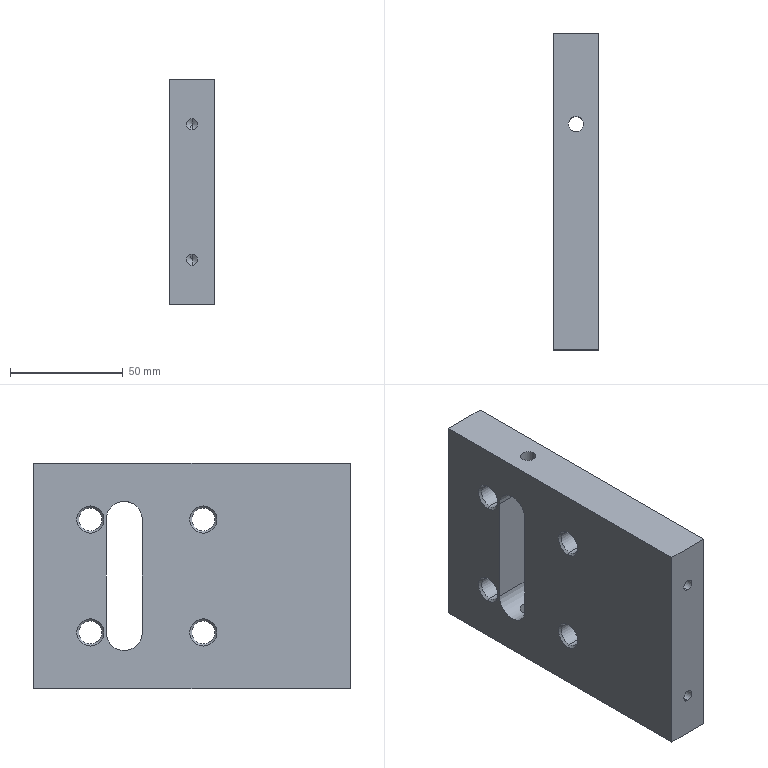Part | SolidWorks | features HoleWzd 4, Extrusion 1, ICE 1 | 1 solid | 47 faces | box 20 x 140 x 100 mm | volume 250918 mm3 | cylinder 23 | cone 16 | plane 8 | commonest cylinder face diameters 5 x8 10.2 x8 6.8 x4 16 x3
STEP:
#1=CARTESIAN_POINT('',(10.,55.,-32.5));
#2=VERTEX_POINT('',#1);
#3=CARTESIAN_POINT('',(10.,55.,-27.5));
#4=VERTEX_POINT('',#3);
#5=CARTESIAN_POINT('',(10.,55.,-30.));
#6=DIRECTION('',(0.,1.,0.));
#7=DIRECTION('',(0.,0.,1.));
#8=AXIS2_PLACEMENT_3D('',#5,#6,#7);
#9=CIRCLE('',#8,2.5);
#10=EDGE_CURVE('',#2,#4,#9,.T.);
#11=ORIENTED_EDGE('',*,*,#10,.F.);
#12=CARTESIAN_POINT('',(10.,70.,-32.5));
#13=VERTEX_POINT('',#12);
#14=CARTESIAN_POINT('',(10.,70.,-32.5));
#15=DIRECTION('',(0.,1.,0.));
#16=VECTOR('',#15,1000.);
#17=LINE('',#14,#16);
#18=EDGE_CURVE('',#2,#13,#17,.T.);
#19=ORIENTED_EDGE('',*,*,#18,.T.);
#20=CARTESIAN_POINT('',(10.,70.,-27.5));
#21=VERTEX_POINT('',#20);
#22=CARTESIAN_POINT('',(10.,70.,-30.));
#23=DIRECTION('',(0.,1.,0.));
#24=DIRECTION('',(0.,0.,1.));
#25=AXIS2_PLACEMENT_3D('',#22,#23,#24);
#26=CIRCLE('',#25,2.5);
#27=EDGE_CURVE('',#13,#21,#26,.T.);
#28=ORIENTED_EDGE('',*,*,#27,.T.);
#29=CARTESIAN_POINT('',(10.,70.,-27.5));
#30=DIRECTION('',(0.,1.,0.));
#31=VECTOR('',#30,1000.);
#32=LINE('',#29,#31);
#33=EDGE_CURVE('',#4,#21,#32,.T.);
#34=ORIENTED_EDGE('',*,*,#33,.F.);
#35=EDGE_LOOP('',(#11,#19,#28,#34));
#36=FACE_OUTER_BOUND('',#35,.T.);
#37=CARTESIAN_POINT('',(10.,70.,-30.));
#38=DIRECTION('',(0.,1.,0.));
#39=DIRECTION('',(0.,0.,1.));
#40=AXIS2_PLACEMENT_3D('',#37,#38,#39);
#41=CYLINDRICAL_SURFACE('',#40,2.5);
#42=ADVANCED_FACE('',(#36),#41,.F.);
#43=CARTESIAN_POINT('',(10.,53.498,-30.));
#44=VERTEX_POINT('',#43);
#45=CARTESIAN_POINT('',(10.,55.,-27.5));
#46=DIRECTION('',(0.,0.515,0.8572));
#47=VECTOR('',#46,1000.);
#48=LINE('',#45,#47);
#49=EDGE_CURVE('',#44,#4,#48,.T.);
#50=ORIENTED_EDGE('',*,*,#49,.F.);
#51=CARTESIAN_POINT('',(10.,55.,-32.5));
#52=DIRECTION('',(0.,0.515,-0.8572));
#53=VECTOR('',#52,1000.);
#54=LINE('',#51,#53);
#55=EDGE_CURVE('',#44,#2,#54,.T.);
#56=ORIENTED_EDGE('',*,*,#55,.T.);
#57=ORIENTED_EDGE('',*,*,#10,.T.);
#58=EDGE_LOOP('',(#50,#56,#57));
#59=FACE_OUTER_BOUND('',#58,.T.);
#60=CARTESIAN_POINT('',(10.,55.,-30.));
#61=DIRECTION('',(0.,1.,0.));
#62=DIRECTION('',(0.,0.,1.));
#63=AXIS2_PLACEMENT_3D('',#60,#61,#62);
#64=CONICAL_SURFACE('',#63,2.5,1.03);
#65=ADVANCED_FACE('',(#59),#64,.F.);
#66=CARTESIAN_POINT('',(10.,55.,27.5));
#67=VERTEX_POINT('',#66);
#68=CARTESIAN_POINT('',(10.,55.,32.5));
#69=VERTEX_POINT('',#68);
#70=CARTESIAN_POINT('',(10.,55.,30.));
#71=DIRECTION('',(0.,1.,0.));
#72=DIRECTION('',(0.,0.,1.));
#73=AXIS2_PLACEMENT_3D('',#70,#71,#72);
#74=CIRCLE('',#73,2.5);
#75=EDGE_CURVE('',#67,#69,#74,.T.);
#76=ORIENTED_EDGE('',*,*,#75,.F.);
#77=CARTESIAN_POINT('',(10.,70.,27.5));
#78=VERTEX_POINT('',#77);
#79=CARTESIAN_POINT('',(10.,70.,27.5));
#80=DIRECTION('',(0.,1.,0.));
#81=VECTOR('',#80,1000.);
#82=LINE('',#79,#81);
#83=EDGE_CURVE('',#67,#78,#82,.T.);
#84=ORIENTED_EDGE('',*,*,#83,.T.);
#85=CARTESIAN_POINT('',(10.,70.,32.5));
#86=VERTEX_POINT('',#85);
#87=CARTESIAN_POINT('',(10.,70.,30.));
#88=DIRECTION('',(0.,1.,0.));
#89=DIRECTION('',(0.,0.,1.));
#90=AXIS2_PLACEMENT_3D('',#87,#88,#89);
#91=CIRCLE('',#90,2.5);
#92=EDGE_CURVE('',#78,#86,#91,.T.);
#93=ORIENTED_EDGE('',*,*,#92,.T.);
#94=CARTESIAN_POINT('',(10.,70.,32.5));
#95=DIRECTION('',(0.,1.,0.));
#96=VECTOR('',#95,1000.);
#97=LINE('',#94,#96);
#98=EDGE_CURVE('',#69,#86,#97,.T.);
#99=ORIENTED_EDGE('',*,*,#98,.F.);
#100=EDGE_LOOP('',(#76,#84,#93,#99));
#101=FACE_OUTER_BOUND('',#100,.T.);
#102=CARTESIAN_POINT('',(10.,70.,30.));
#103=DIRECTION('',(0.,1.,0.));
#104=DIRECTION('',(0.,0.,1.));
#105=AXIS2_PLACEMENT_3D('',#102,#103,#104);
#106=CYLINDRICAL_SURFACE('',#105,2.5);
#107=ADVANCED_FACE('',(#101),#106,.F.);
#108=CARTESIAN_POINT('',(10.,53.498,30.));
#109=VERTEX_POINT('',#108);
#110=CARTESIAN_POINT('',(10.,55.,32.5));
#111=DIRECTION('',(0.,0.515,0.8572));
#112=VECTOR('',#111,1000.);
#113=LINE('',#110,#112);
#114=EDGE_CURVE('',#109,#69,#113,.T.);
#115=ORIENTED_EDGE('',*,*,#114,.F.);
#116=CARTESIAN_POINT('',(10.,55.,27.5));
#117=DIRECTION('',(0.,0.515,-0.8572));
#118=VECTOR('',#117,1000.);
#119=LINE('',#116,#118);
#120=EDGE_CURVE('',#109,#67,#119,.T.);
#121=ORIENTED_EDGE('',*,*,#120,.T.);
#122=ORIENTED_EDGE('',*,*,#75,.T.);
#123=EDGE_LOOP('',(#115,#121,#122));
#124=FACE_OUTER_BOUND('',#123,.T.);
#125=CARTESIAN_POINT('',(10.,55.,30.));
#126=DIRECTION('',(0.,1.,0.));
#127=DIRECTION('',(0.,0.,1.));
#128=AXIS2_PLACEMENT_3D('',#125,#126,#127);
#129=CONICAL_SURFACE('',#128,2.5,1.03);
#130=ADVANCED_FACE('',(#124),#129,.F.);
#131=CARTESIAN_POINT('',(0.925,45.,-30.1));
#132=VERTEX_POINT('',#131);
#133=CARTESIAN_POINT('',(0.925,45.,-19.9));
#134=VERTEX_POINT('',#133);
#135=CARTESIAN_POINT('',(0.925,45.,-25.));
#136=DIRECTION('',(-1.,0.,0.));
#137=DIRECTION('',(0.,0.,1.));
#138=AXIS2_PLACEMENT_3D('',#135,#136,#137);
#139=CIRCLE('',#138,5.1);
#140=EDGE_CURVE('',#132,#134,#139,.T.);
#141=ORIENTED_EDGE('',*,*,#140,.F.);
#142=CARTESIAN_POINT('',(0.,45.,-31.025));
#143=VERTEX_POINT('',#142);
#144=CARTESIAN_POINT('',(0.,45.,-31.025));
#145=DIRECTION('',(-0.7071,0.,-0.7071));
#146=VECTOR('',#145,1000.);
#147=LINE('',#144,#146);
#148=EDGE_CURVE('',#132,#143,#147,.T.);
#149=ORIENTED_EDGE('',*,*,#148,.T.);
#150=CARTESIAN_POINT('',(0.,45.,-18.975));
#151=VERTEX_POINT('',#150);
#152=CARTESIAN_POINT('',(0.,45.,-25.));
#153=DIRECTION('',(-1.,0.,0.));
#154=DIRECTION('',(0.,0.,1.));
#155=AXIS2_PLACEMENT_3D('',#152,#153,#154);
#156=CIRCLE('',#155,6.025);
#157=EDGE_CURVE('',#143,#151,#156,.T.);
#158=ORIENTED_EDGE('',*,*,#157,.T.);
#159=CARTESIAN_POINT('',(0.,45.,-18.975));
#160=DIRECTION('',(-0.7071,0.,0.7071));
#161=VECTOR('',#160,1000.);
#162=LINE('',#159,#161);
#163=EDGE_CURVE('',#134,#151,#162,.T.);
#164=ORIENTED_EDGE('',*,*,#163,.F.);
#165=EDGE_LOOP('',(#141,#149,#158,#164));
#166=FACE_OUTER_BOUND('',#165,.T.);
#167=CARTESIAN_POINT('',(0.,45.,-25.));
#168=DIRECTION('',(-1.,0.,0.));
#169=DIRECTION('',(0.,0.,1.));
#170=AXIS2_PLACEMENT_3D('',#167,#168,#169);
#171=CONICAL_SURFACE('',#170,6.025,0.7854);
#172=ADVANCED_FACE('',(#166),#171,.F.);
#173=CARTESIAN_POINT('',(20.,45.,-30.1));
#174=VERTEX_POINT('',#173);
#175=CARTESIAN_POINT('',(20.,45.,-19.9));
#176=VERTEX_POINT('',#175);
#177=CARTESIAN_POINT('',(20.,45.,-25.));
#178=DIRECTION('',(-1.,0.,0.));
#179=DIRECTION('',(0.,0.,1.));
#180=AXIS2_PLACEMENT_3D('',#177,#178,#179);
#181=CIRCLE('',#180,5.1);
#182=EDGE_CURVE('',#174,#176,#181,.T.);
#183=ORIENTED_EDGE('',*,*,#182,.F.);
#184=CARTESIAN_POINT('',(0.,45.,-30.1));
#185=DIRECTION('',(-1.,0.,0.));
#186=VECTOR('',#185,1000.);
#187=LINE('',#184,#186);
#188=EDGE_CURVE('',#174,#132,#187,.T.);
#189=ORIENTED_EDGE('',*,*,#188,.T.);
#190=ORIENTED_EDGE('',*,*,#140,.T.);
#191=CARTESIAN_POINT('',(0.,45.,-19.9));
#192=DIRECTION('',(-1.,0.,0.));
#193=VECTOR('',#192,1000.);
#194=LINE('',#191,#193);
#195=EDGE_CURVE('',#176,#134,#194,.T.);
#196=ORIENTED_EDGE('',*,*,#195,.F.);
#197=EDGE_LOOP('',(#183,#189,#190,#196));
#198=FACE_OUTER_BOUND('',#197,.T.);
#199=CARTESIAN_POINT('',(0.,45.,-25.));
#200=DIRECTION('',(-1.,0.,0.));
#201=DIRECTION('',(0.,0.,1.));
#202=AXIS2_PLACEMENT_3D('',#199,#200,#201);
#203=CYLINDRICAL_SURFACE('',#202,5.1);
#204=ADVANCED_FACE('',(#198),#203,.F.);
#205=CARTESIAN_POINT('',(0.925,45.,19.9));
#206=VERTEX_POINT('',#205);
#207=CARTESIAN_POINT('',(0.925,45.,30.1));
#208=VERTEX_POINT('',#207);
#209=CARTESIAN_POINT('',(0.925,45.,25.));
#210=DIRECTION('',(-1.,0.,0.));
#211=DIRECTION('',(0.,0.,1.));
#212=AXIS2_PLACEMENT_3D('',#209,#210,#211);
#213=CIRCLE('',#212,5.1);
#214=EDGE_CURVE('',#206,#208,#213,.T.);
#215=ORIENTED_EDGE('',*,*,#214,.F.);
#216=CARTESIAN_POINT('',(0.,45.,18.975));
#217=VERTEX_POINT('',#216);
#218=CARTESIAN_POINT('',(0.,45.,18.975));
#219=DIRECTION('',(-0.7071,0.,-0.7071));
#220=VECTOR('',#219,1000.);
#221=LINE('',#218,#220);
#222=EDGE_CURVE('',#206,#217,#221,.T.);
#223=ORIENTED_EDGE('',*,*,#222,.T.);
#224=CARTESIAN_POINT('',(0.,45.,31.025));
#225=VERTEX_POINT('',#224);
#226=CARTESIAN_POINT('',(0.,45.,25.));
#227=DIRECTION('',(-1.,0.,0.));
#228=DIRECTION('',(0.,0.,1.));
#229=AXIS2_PLACEMENT_3D('',#226,#227,#228);
#230=CIRCLE('',#229,6.025);
#231=EDGE_CURVE('',#217,#225,#230,.T.);
#232=ORIENTED_EDGE('',*,*,#231,.T.);
#233=CARTESIAN_POINT('',(0.,45.,31.025));
#234=DIRECTION('',(-0.7071,0.,0.7071));
#235=VECTOR('',#234,1000.);
#236=LINE('',#233,#235);
#237=EDGE_CURVE('',#208,#225,#236,.T.);
#238=ORIENTED_EDGE('',*,*,#237,.F.);
#239=EDGE_LOOP('',(#215,#223,#232,#238));
#240=FACE_OUTER_BOUND('',#239,.T.);
#241=CARTESIAN_POINT('',(0.,45.,25.));
#242=DIRECTION('',(-1.,0.,0.));
#243=DIRECTION('',(0.,0.,1.));
#244=AXIS2_PLACEMENT_3D('',#241,#242,#243);
#245=CONICAL_SURFACE('',#244,6.025,0.7854);
#246=ADVANCED_FACE('',(#240),#245,.F.);
#247=CARTESIAN_POINT('',(20.,45.,19.9));
#248=VERTEX_POINT('',#247);
#249=CARTESIAN_POINT('',(20.,45.,30.1));
#250=VERTEX_POINT('',#249);
#251=CARTESIAN_POINT('',(20.,45.,25.));
#252=DIRECTION('',(-1.,0.,0.));
#253=DIRECTION('',(0.,0.,1.));
#254=AXIS2_PLACEMENT_3D('',#251,#252,#253);
#255=CIRCLE('',#254,5.1);
#256=EDGE_CURVE('',#248,#250,#255,.T.);
#257=ORIENTED_EDGE('',*,*,#256,.F.);
#258=CARTESIAN_POINT('',(0.,45.,19.9));
#259=DIRECTION('',(-1.,0.,0.));
#260=VECTOR('',#259,1000.);
#261=LINE('',#258,#260);
#262=EDGE_CURVE('',#248,#206,#261,.T.);
#263=ORIENTED_EDGE('',*,*,#262,.T.);
#264=ORIENTED_EDGE('',*,*,#214,.T.);
#265=CARTESIAN_POINT('',(0.,45.,30.1));
#266=DIRECTION('',(-1.,0.,0.));
#267=VECTOR('',#266,1000.);
#268=LINE('',#265,#267);
#269=EDGE_CURVE('',#250,#208,#268,.T.);
#270=ORIENTED_EDGE('',*,*,#269,.F.);
#271=EDGE_LOOP('',(#257,#263,#264,#270));
#272=FACE_OUTER_BOUND('',#271,.T.);
#273=CARTESIAN_POINT('',(0.,45.,25.));
#274=DIRECTION('',(-1.,0.,0.));
#275=DIRECTION('',(0.,0.,1.));
#276=AXIS2_PLACEMENT_3D('',#273,#274,#275);
#277=CYLINDRICAL_SURFACE('',#276,5.1);
#278=ADVANCED_FACE('',(#272),#277,.F.);
#279=CARTESIAN_POINT('',(0.925,-5.,-30.1));
#280=VERTEX_POINT('',#279);
#281=CARTESIAN_POINT('',(0.925,-5.,-19.9));
#282=VERTEX_POINT('',#281);
#283=CARTESIAN_POINT('',(0.925,-5.,-25.));
#284=DIRECTION('',(-1.,0.,0.));
#285=DIRECTION('',(0.,0.,1.));
#286=AXIS2_PLACEMENT_3D('',#283,#284,#285);
#287=CIRCLE('',#286,5.1);
#288=EDGE_CURVE('',#280,#282,#287,.T.);
#289=ORIENTED_EDGE('',*,*,#288,.F.);
#290=CARTESIAN_POINT('',(0.,-5.,-31.025));
#291=VERTEX_POINT('',#290);
#292=CARTESIAN_POINT('',(0.,-5.,-31.025));
#293=DIRECTION('',(-0.7071,0.,-0.7071));
#294=VECTOR('',#293,1000.);
#295=LINE('',#292,#294);
#296=EDGE_CURVE('',#280,#291,#295,.T.);
#297=ORIENTED_EDGE('',*,*,#296,.T.);
#298=CARTESIAN_POINT('',(0.,-5.,-18.975));
#299=VERTEX_POINT('',#298);
#300=CARTESIAN_POINT('',(0.,-5.,-25.));
#301=DIRECTION('',(-1.,0.,0.));
#302=DIRECTION('',(0.,0.,1.));
#303=AXIS2_PLACEMENT_3D('',#300,#301,#302);
#304=CIRCLE('',#303,6.025);
#305=EDGE_CURVE('',#291,#299,#304,.T.);
#306=ORIENTED_EDGE('',*,*,#305,.T.);
#307=CARTESIAN_POINT('',(0.,-5.,-18.975));
#308=DIRECTION('',(-0.7071,0.,0.7071));
#309=VECTOR('',#308,1000.);
#310=LINE('',#307,#309);
#311=EDGE_CURVE('',#282,#299,#310,.T.);
#312=ORIENTED_EDGE('',*,*,#311,.F.);
#313=EDGE_LOOP('',(#289,#297,#306,#312));
#314=FACE_OUTER_BOUND('',#313,.T.);
#315=CARTESIAN_POINT('',(0.,-5.,-25.));
#316=DIRECTION('',(-1.,0.,0.));
#317=DIRECTION('',(0.,0.,1.));
#318=AXIS2_PLACEMENT_3D('',#315,#316,#317);
#319=CONICAL_SURFACE('',#318,6.025,0.7854);
#320=ADVANCED_FACE('',(#314),#319,.F.);
#321=CARTESIAN_POINT('',(20.,-5.,-30.1));
#322=VERTEX_POINT('',#321);
#323=CARTESIAN_POINT('',(20.,-5.,-19.9));
#324=VERTEX_POINT('',#323);
#325=CARTESIAN_POINT('',(20.,-5.,-25.));
#326=DIRECTION('',(-1.,0.,0.));
#327=DIRECTION('',(0.,0.,1.));
#328=AXIS2_PLACEMENT_3D('',#325,#326,#327);
#329=CIRCLE('',#328,5.1);
#330=EDGE_CURVE('',#322,#324,#329,.T.);
#331=ORIENTED_EDGE('',*,*,#330,.F.);
#332=CARTESIAN_POINT('',(0.,-5.,-30.1));
#333=DIRECTION('',(-1.,0.,0.));
#334=VECTOR('',#333,1000.);
#335=LINE('',#332,#334);
#336=EDGE_CURVE('',#322,#280,#335,.T.);
#337=ORIENTED_EDGE('',*,*,#336,.T.);
#338=ORIENTED_EDGE('',*,*,#288,.T.);
#339=CARTESIAN_POINT('',(0.,-5.,-19.9));
#340=DIRECTION('',(-1.,0.,0.));
#341=VECTOR('',#340,1000.);
#342=LINE('',#339,#341);
#343=EDGE_CURVE('',#324,#282,#342,.T.);
#344=ORIENTED_EDGE('',*,*,#343,.F.);
#345=EDGE_LOOP('',(#331,#337,#338,#344));
#346=FACE_OUTER_BOUND('',#345,.T.);
#347=CARTESIAN_POINT('',(0.,-5.,-25.));
#348=DIRECTION('',(-1.,0.,0.));
#349=DIRECTION('',(0.,0.,1.));
#350=AXIS2_PLACEMENT_3D('',#347,#348,#349);
#351=CYLINDRICAL_SURFACE('',#350,5.1);
#352=ADVANCED_FACE('',(#346),#351,.F.);
#353=CARTESIAN_POINT('',(0.925,-5.,19.9));
#354=VERTEX_POINT('',#353);
#355=CARTESIAN_POINT('',(0.925,-5.,30.1));
#356=VERTEX_POINT('',#355);
#357=CARTESIAN_POINT('',(0.925,-5.,25.));
#358=DIRECTION('',(-1.,0.,0.));
#359=DIRECTION('',(0.,0.,1.));
#360=AXIS2_PLACEMENT_3D('',#357,#358,#359);
#361=CIRCLE('',#360,5.1);
#362=EDGE_CURVE('',#354,#356,#361,.T.);
#363=ORIENTED_EDGE('',*,*,#362,.F.);
#364=CARTESIAN_POINT('',(0.,-5.,18.975));
#365=VERTEX_POINT('',#364);
#366=CARTESIAN_POINT('',(0.,-5.,18.975));
#367=DIRECTION('',(-0.7071,0.,-0.7071));
#368=VECTOR('',#367,1000.);
#369=LINE('',#366,#368);
#370=EDGE_CURVE('',#354,#365,#369,.T.);
#371=ORIENTED_EDGE('',*,*,#370,.T.);
#372=CARTESIAN_POINT('',(0.,-5.,31.025));
#373=VERTEX_POINT('',#372);
#374=CARTESIAN_POINT('',(0.,-5.,25.));
#375=DIRECTION('',(-1.,0.,0.));
#376=DIRECTION('',(0.,0.,1.));
#377=AXIS2_PLACEMENT_3D('',#374,#375,#376);
#378=CIRCLE('',#377,6.025);
#379=EDGE_CURVE('',#365,#373,#378,.T.);
#380=ORIENTED_EDGE('',*,*,#379,.T.);
#381=CARTESIAN_POINT('',(0.,-5.,31.025));
#382=DIRECTION('',(-0.7071,0.,0.7071));
#383=VECTOR('',#382,1000.);
#384=LINE('',#381,#383);
#385=EDGE_CURVE('',#356,#373,#384,.T.);
#386=ORIENTED_EDGE('',*,*,#385,.F.);
#387=EDGE_LOOP('',(#363,#371,#380,#386));
#388=FACE_OUTER_BOUND('',#387,.T.);
#389=CARTESIAN_POINT('',(0.,-5.,25.));
#390=DIRECTION('',(-1.,0.,0.));
#391=DIRECTION('',(0.,0.,1.));
#392=AXIS2_PLACEMENT_3D('',#389,#390,#391);
#393=CONICAL_SURFACE('',#392,6.025,0.7854);
#394=ADVANCED_FACE('',(#388),#393,.F.);
#395=CARTESIAN_POINT('',(20.,-5.,19.9));
#396=VERTEX_POINT('',#395);
#397=CARTESIAN_POINT('',(20.,-5.,30.1));
#398=VERTEX_POINT('',#397);
#399=CARTESIAN_POINT('',(20.,-5.,25.));
#400=DIRECTION('',(-1.,0.,0.));
#401=DIRECTION('',(0.,0.,1.));
#402=AXIS2_PLACEMENT_3D('',#399,#400,#401);
#403=CIRCLE('',#402,5.1);
#404=EDGE_CURVE('',#396,#398,#403,.T.);
#405=ORIENTED_EDGE('',*,*,#404,.F.);
#406=CARTESIAN_POINT('',(0.,-5.,19.9));
#407=DIRECTION('',(-1.,0.,0.));
#408=VECTOR('',#407,1000.);
#409=LINE('',#406,#408);
#410=EDGE_CURVE('',#396,#354,#409,.T.);
#411=ORIENTED_EDGE('',*,*,#410,.T.);
#412=ORIENTED_EDGE('',*,*,#362,.T.);
#413=CARTESIAN_POINT('',(0.,-5.,30.1));
#414=DIRECTION('',(-1.,0.,0.));
#415=VECTOR('',#414,1000.);
#416=LINE('',#413,#415);
#417=EDGE_CURVE('',#398,#356,#416,.T.);
#418=ORIENTED_EDGE('',*,*,#417,.F.);
#419=EDGE_LOOP('',(#405,#411,#412,#418));
#420=FACE_OUTER_BOUND('',#419,.T.);
#421=CARTESIAN_POINT('',(0.,-5.,25.));
#422=DIRECTION('',(-1.,0.,0.));
#423=DIRECTION('',(0.,0.,1.));
#424=AXIS2_PLACEMENT_3D('',#421,#422,#423);
#425=CYLINDRICAL_SURFACE('',#424,5.1);
#426=ADVANCED_FACE('',(#420),#425,.F.);
#427=CARTESIAN_POINT('',(6.6,30.,-50.));
#428=VERTEX_POINT('',#427);
#429=CARTESIAN_POINT('',(13.4,30.,-50.));
#430=VERTEX_POINT('',#429);
#431=CARTESIAN_POINT('',(10.,30.,-50.));
#432=DIRECTION('',(0.,0.,1.));
#433=DIRECTION('',(1.,0.,0.));
#434=AXIS2_PLACEMENT_3D('',#431,#432,#433);
#435=CIRCLE('',#434,3.4);
#436=EDGE_CURVE('',#428,#430,#435,.T.);
#437=ORIENTED_EDGE('',*,*,#436,.F.);
#438=CARTESIAN_POINT('',(6.6,30.,-33.));
#439=VERTEX_POINT('',#438);
#440=CARTESIAN_POINT('',(6.6,30.,50.));
#441=DIRECTION('',(0.,0.,1.));
#442=VECTOR('',#441,1000.);
#443=LINE('',#440,#442);
#444=EDGE_CURVE('',#428,#439,#443,.T.);
#445=ORIENTED_EDGE('',*,*,#444,.T.);
#446=CARTESIAN_POINT('',(13.4,30.,-33.));
#447=VERTEX_POINT('',#446);
#448=CARTESIAN_POINT('',(13.4,30.,-33.));
#449=CARTESIAN_POINT('',(13.4,29.772,-33.));
#450=CARTESIAN_POINT('',(13.377,29.549,-32.99));
#451=CARTESIAN_POINT('',(13.289,29.111,-32.953));
#452=CARTESIAN_POINT('',(13.223,28.893,-32.926));
#453=CARTESIAN_POINT('',(13.051,28.483,-32.858));
#454=CARTESIAN_POINT('',(12.946,28.288,-32.817));
#455=CARTESIAN_POINT('',(12.699,27.92,-32.727));
#456=CARTESIAN_POINT('',(12.557,27.749,-32.678));
#457=CARTESIAN_POINT('',(12.247,27.439,-32.581));
#458=CARTESIAN_POINT('',(12.077,27.299,-32.531));
#459=CARTESIAN_POINT('',(11.708,27.052,-32.438));
#460=CARTESIAN_POINT('',(11.514,26.948,-32.395));
#461=CARTESIAN_POINT('',(11.107,26.778,-32.323));
#462=CARTESIAN_POINT('',(10.89,26.711,-32.293));
#463=CARTESIAN_POINT('',(10.45,26.622,-32.252));
#464=CARTESIAN_POINT('',(10.227,26.6,-32.242));
#465=CARTESIAN_POINT('',(9.777,26.6,-32.241));
#466=CARTESIAN_POINT('',(9.549,26.623,-32.252));
#467=CARTESIAN_POINT('',(9.111,26.711,-32.293));
#468=CARTESIAN_POINT('',(8.896,26.776,-32.322));
#469=CARTESIAN_POINT('',(8.483,26.949,-32.396));
#470=CARTESIAN_POINT('',(8.289,27.054,-32.439));
#471=CARTESIAN_POINT('',(7.923,27.299,-32.531));
#472=CARTESIAN_POINT('',(7.75,27.441,-32.582));
#473=CARTESIAN_POINT('',(7.44,27.752,-32.679));
#474=CARTESIAN_POINT('',(7.301,27.921,-32.727));
#475=CARTESIAN_POINT('',(7.054,28.289,-32.817));
#476=CARTESIAN_POINT('',(6.948,28.486,-32.858));
#477=CARTESIAN_POINT('',(6.777,28.895,-32.926));
#478=CARTESIAN_POINT('',(6.711,29.108,-32.953));
#479=CARTESIAN_POINT('',(6.622,29.552,-32.991));
#480=CARTESIAN_POINT('',(6.6,29.776,-33.));
#481=CARTESIAN_POINT('',(6.6,30.,-33.));
#482=B_SPLINE_CURVE_WITH_KNOTS('',3,(#448,#449,#450,#451,#452,#453,#454,#455,#456,#457,#458,#459,#460,#461,#462,#463,#464,#465,#466,#467,#468,#469,#470,#471,#472,#473,#474,#475,#476,#477,#478,#479,#480,#481),.UNSPECIFIED.,.F.,.F.,(4,2,2,2,2,2,2,2,2,2,2,2,2,2,2,2,4),(0.,0.0006725,0.001345,0.002017,0.00269,0.003362,0.004035,0.004707,0.00538,0.006052,0.006725,0.007397,0.00807,0.008742,0.009415,0.01009,0.01076),.UNSPECIFIED.);
#483=EDGE_CURVE('',#447,#439,#482,.T.);
#484=ORIENTED_EDGE('',*,*,#483,.F.);
#485=CARTESIAN_POINT('',(13.4,30.,50.));
#486=DIRECTION('',(0.,0.,1.));
#487=VECTOR('',#486,1000.);
#488=LINE('',#485,#487);
#489=EDGE_CURVE('',#430,#447,#488,.T.);
#490=ORIENTED_EDGE('',*,*,#489,.F.);
#491=EDGE_LOOP('',(#437,#445,#484,#490));
#492=FACE_OUTER_BOUND('',#491,.T.);
#493=CARTESIAN_POINT('',(10.,30.,50.));
#494=DIRECTION('',(0.,0.,1.));
#495=DIRECTION('',(1.,0.,0.));
#496=AXIS2_PLACEMENT_3D('',#493,#494,#495);
#497=CYLINDRICAL_SURFACE('',#496,3.4);
#498=ADVANCED_FACE('',(#492),#497,.F.);
#499=CARTESIAN_POINT('',(6.6,30.,33.));
#500=VERTEX_POINT('',#499);
#501=CARTESIAN_POINT('',(13.4,30.,33.));
#502=VERTEX_POINT('',#501);
#503=CARTESIAN_POINT('',(6.6,30.,33.));
#504=CARTESIAN_POINT('',(6.6,29.776,33.));
#505=CARTESIAN_POINT('',(6.623,29.549,32.99));
#506=CARTESIAN_POINT('',(6.711,29.108,32.953));
#507=CARTESIAN_POINT('',(6.777,28.895,32.926));
#508=CARTESIAN_POINT('',(6.949,28.483,32.858));
#509=CARTESIAN_POINT('',(7.055,28.286,32.816));
#510=CARTESIAN_POINT('',(7.301,27.921,32.727));
#511=CARTESIAN_POINT('',(7.442,27.75,32.679));
#512=CARTESIAN_POINT('',(7.754,27.438,32.58));
#513=CARTESIAN_POINT('',(7.924,27.299,32.531));
#514=CARTESIAN_POINT('',(8.288,27.054,32.439));
#515=CARTESIAN_POINT('',(8.486,26.947,32.395));
#516=CARTESIAN_POINT('',(8.896,26.777,32.322));
#517=CARTESIAN_POINT('',(9.108,26.712,32.293));
#518=CARTESIAN_POINT('',(9.547,26.623,32.252));
#519=CARTESIAN_POINT('',(9.775,26.6,32.242));
#520=CARTESIAN_POINT('',(10.223,26.6,32.242));
#521=CARTESIAN_POINT('',(10.446,26.622,32.252));
#522=CARTESIAN_POINT('',(10.891,26.711,32.293));
#523=CARTESIAN_POINT('',(11.104,26.776,32.322));
#524=CARTESIAN_POINT('',(11.513,26.947,32.395));
#525=CARTESIAN_POINT('',(11.711,27.054,32.439));
#526=CARTESIAN_POINT('',(12.077,27.299,32.531));
#527=CARTESIAN_POINT('',(12.247,27.438,32.581));
#528=CARTESIAN_POINT('',(12.559,27.75,32.679));
#529=CARTESIAN_POINT('',(12.7,27.922,32.728));
#530=CARTESIAN_POINT('',(12.945,28.286,32.817));
#531=CARTESIAN_POINT('',(13.05,28.482,32.857));
#532=CARTESIAN_POINT('',(13.223,28.896,32.926));
#533=CARTESIAN_POINT('',(13.289,29.108,32.953));
#534=CARTESIAN_POINT('',(13.377,29.546,32.99));
#535=CARTESIAN_POINT('',(13.4,29.773,33.));
#536=CARTESIAN_POINT('',(13.4,30.,33.));
#537=B_SPLINE_CURVE_WITH_KNOTS('',3,(#503,#504,#505,#506,#507,#508,#509,#510,#511,#512,#513,#514,#515,#516,#517,#518,#519,#520,#521,#522,#523,#524,#525,#526,#527,#528,#529,#530,#531,#532,#533,#534,#535,#536),.UNSPECIFIED.,.F.,.F.,(4,2,2,2,2,2,2,2,2,2,2,2,2,2,2,2,4),(0.01076,0.01143,0.0121,0.01278,0.01345,0.01412,0.01479,0.01546,0.01613,0.01681,0.01748,0.01815,0.01882,0.01949,0.02017,0.02084,0.02151),.UNSPECIFIED.);
#538=EDGE_CURVE('',#500,#502,#537,.T.);
#539=ORIENTED_EDGE('',*,*,#538,.F.);
#540=CARTESIAN_POINT('',(6.6,30.,50.));
#541=VERTEX_POINT('',#540);
#542=CARTESIAN_POINT('',(6.6,30.,50.));
#543=DIRECTION('',(0.,0.,1.));
#544=VECTOR('',#543,1000.);
#545=LINE('',#542,#544);
#546=EDGE_CURVE('',#500,#541,#545,.T.);
#547=ORIENTED_EDGE('',*,*,#546,.T.);
#548=CARTESIAN_POINT('',(13.4,30.,50.));
#549=VERTEX_POINT('',#548);
#550=CARTESIAN_POINT('',(10.,30.,50.));
#551=DIRECTION('',(0.,0.,1.));
#552=DIRECTION('',(1.,0.,0.));
#553=AXIS2_PLACEMENT_3D('',#550,#551,#552);
#554=CIRCLE('',#553,3.4);
#555=EDGE_CURVE('',#541,#549,#554,.T.);
#556=ORIENTED_EDGE('',*,*,#555,.T.);
#557=CARTESIAN_POINT('',(13.4,30.,50.));
#558=DIRECTION('',(0.,0.,1.));
#559=VECTOR('',#558,1000.);
#560=LINE('',#557,#559);
#561=EDGE_CURVE('',#502,#549,#560,.T.);
#562=ORIENTED_EDGE('',*,*,#561,.F.);
#563=EDGE_LOOP('',(#539,#547,#556,#562));
#564=FACE_OUTER_BOUND('',#563,.T.);
#565=CARTESIAN_POINT('',(10.,30.,50.));
#566=DIRECTION('',(0.,0.,1.));
#567=DIRECTION('',(1.,0.,0.));
#568=AXIS2_PLACEMENT_3D('',#565,#566,#567);
#569=CYLINDRICAL_SURFACE('',#568,3.4);
#570=ADVANCED_FACE('',(#564),#569,.F.);
#571=CARTESIAN_POINT('',(20.,30.,33.));
#572=VERTEX_POINT('',#571);
#573=CARTESIAN_POINT('',(20.,38.,25.));
#574=VERTEX_POINT('',#573);
#575=CARTESIAN_POINT('',(20.,30.,25.));
#576=DIRECTION('',(-1.,0.,0.));
#577=DIRECTION('',(0.,0.,1.));
#578=AXIS2_PLACEMENT_3D('',#575,#576,#577);
#579=CIRCLE('',#578,8.);
#580=EDGE_CURVE('',#572,#574,#579,.T.);
#581=ORIENTED_EDGE('',*,*,#580,.F.);
#582=CARTESIAN_POINT('',(20.,30.,33.));
#583=DIRECTION('',(-1.,0.,0.));
#584=VECTOR('',#583,1000.);
#585=LINE('',#582,#584);
#586=EDGE_CURVE('',#572,#502,#585,.T.);
#587=ORIENTED_EDGE('',*,*,#586,.T.);
#588=CARTESIAN_POINT('',(13.4,30.,33.));
#589=CARTESIAN_POINT('',(13.4,30.228,33.));
#590=CARTESIAN_POINT('',(13.377,30.451,32.99));
#591=CARTESIAN_POINT('',(13.289,30.889,32.953));
#592=CARTESIAN_POINT('',(13.223,31.107,32.926));
#593=CARTESIAN_POINT('',(13.051,31.517,32.858));
#594=CARTESIAN_POINT('',(12.946,31.712,32.817));
#595=CARTESIAN_POINT('',(12.699,32.08,32.727));
#596=CARTESIAN_POINT('',(12.557,32.251,32.678));
#597=CARTESIAN_POINT('',(12.247,32.561,32.581));
#598=CARTESIAN_POINT('',(12.077,32.701,32.531));
#599=CARTESIAN_POINT('',(11.708,32.948,32.438));
#600=CARTESIAN_POINT('',(11.514,33.052,32.395));
#601=CARTESIAN_POINT('',(11.107,33.222,32.323));
#602=CARTESIAN_POINT('',(10.89,33.289,32.293));
#603=CARTESIAN_POINT('',(10.45,33.378,32.252));
#604=CARTESIAN_POINT('',(10.227,33.4,32.242));
#605=CARTESIAN_POINT('',(9.777,33.4,32.241));
#606=CARTESIAN_POINT('',(9.549,33.377,32.252));
#607=CARTESIAN_POINT('',(9.111,33.289,32.293));
#608=CARTESIAN_POINT('',(8.896,33.224,32.322));
#609=CARTESIAN_POINT('',(8.483,33.051,32.396));
#610=CARTESIAN_POINT('',(8.289,32.946,32.439));
#611=CARTESIAN_POINT('',(7.923,32.701,32.531));
#612=CARTESIAN_POINT('',(7.75,32.559,32.582));
#613=CARTESIAN_POINT('',(7.44,32.248,32.679));
#614=CARTESIAN_POINT('',(7.301,32.079,32.727));
#615=CARTESIAN_POINT('',(7.054,31.711,32.817));
#616=CARTESIAN_POINT('',(6.948,31.514,32.858));
#617=CARTESIAN_POINT('',(6.777,31.105,32.926));
#618=CARTESIAN_POINT('',(6.711,30.892,32.953));
#619=CARTESIAN_POINT('',(6.622,30.448,32.991));
#620=CARTESIAN_POINT('',(6.6,30.224,33.));
#621=CARTESIAN_POINT('',(6.6,30.,33.));
#622=B_SPLINE_CURVE_WITH_KNOTS('',3,(#588,#589,#590,#591,#592,#593,#594,#595,#596,#597,#598,#599,#600,#601,#602,#603,#604,#605,#606,#607,#608,#609,#610,#611,#612,#613,#614,#615,#616,#617,#618,#619,#620,#621),.UNSPECIFIED.,.F.,.F.,(4,2,2,2,2,2,2,2,2,2,2,2,2,2,2,2,4),(0.,0.0006725,0.001345,0.002017,0.00269,0.003362,0.004035,0.004707,0.00538,0.006052,0.006725,0.007397,0.00807,0.008742,0.009415,0.01009,0.01076),.UNSPECIFIED.);
#623=EDGE_CURVE('',#502,#500,#622,.T.);
#624=ORIENTED_EDGE('',*,*,#623,.T.);
#625=CARTESIAN_POINT('',(0.,30.,33.));
#626=VERTEX_POINT('',#625);
#627=CARTESIAN_POINT('',(20.,30.,33.));
#628=DIRECTION('',(-1.,0.,0.));
#629=VECTOR('',#628,1000.);
#630=LINE('',#627,#629);
#631=EDGE_CURVE('',#500,#626,#630,.T.);
#632=ORIENTED_EDGE('',*,*,#631,.T.);
#633=CARTESIAN_POINT('',(0.,38.,25.));
#634=VERTEX_POINT('',#633);
#635=CARTESIAN_POINT('',(0.,30.,25.));
#636=DIRECTION('',(-1.,0.,0.));
#637=DIRECTION('',(0.,0.,1.));
#638=AXIS2_PLACEMENT_3D('',#635,#636,#637);
#639=CIRCLE('',#638,8.);
#640=EDGE_CURVE('',#626,#634,#639,.T.);
#641=ORIENTED_EDGE('',*,*,#640,.T.);
#642=CARTESIAN_POINT('',(20.,38.,25.));
#643=DIRECTION('',(-1.,0.,0.));
#644=VECTOR('',#643,1000.);
#645=LINE('',#642,#644);
#646=EDGE_CURVE('',#574,#634,#645,.T.);
#647=ORIENTED_EDGE('',*,*,#646,.F.);
#648=EDGE_LOOP('',(#581,#587,#624,#632,#641,#647));
#649=FACE_OUTER_BOUND('',#648,.T.);
#650=CARTESIAN_POINT('',(20.,30.,25.));
#651=DIRECTION('',(-1.,0.,0.));
#652=DIRECTION('',(0.,0.,1.));
#653=AXIS2_PLACEMENT_3D('',#650,#651,#652);
#654=CYLINDRICAL_SURFACE('',#653,8.);
#655=ADVANCED_FACE('',(#649),#654,.F.);
#656=CARTESIAN_POINT('',(10.,-55.,-27.5));
#657=VERTEX_POINT('',#656);
#658=CARTESIAN_POINT('',(10.,-55.,-32.5));
#659=VERTEX_POINT('',#658);
#660=CARTESIAN_POINT('',(10.,-55.,-30.));
#661=DIRECTION('',(0.,-1.,0.));
#662=DIRECTION('',(0.,0.,-1.));
#663=AXIS2_PLACEMENT_3D('',#660,#661,#662);
#664=CIRCLE('',#663,2.5);
#665=EDGE_CURVE('',#657,#659,#664,.T.);
#666=ORIENTED_EDGE('',*,*,#665,.F.);
#667=CARTESIAN_POINT('',(10.,-70.,-27.5));
#668=VERTEX_POINT('',#667);
#669=CARTESIAN_POINT('',(10.,-70.,-27.5));
#670=DIRECTION('',(0.,-1.,0.));
#671=VECTOR('',#670,1000.);
#672=LINE('',#669,#671);
#673=EDGE_CURVE('',#657,#668,#672,.T.);
#674=ORIENTED_EDGE('',*,*,#673,.T.);
#675=CARTESIAN_POINT('',(10.,-70.,-32.5));
#676=VERTEX_POINT('',#675);
#677=CARTESIAN_POINT('',(10.,-70.,-30.));
#678=DIRECTION('',(0.,-1.,0.));
#679=DIRECTION('',(0.,0.,-1.));
#680=AXIS2_PLACEMENT_3D('',#677,#678,#679);
#681=CIRCLE('',#680,2.5);
#682=EDGE_CURVE('',#668,#676,#681,.T.);
#683=ORIENTED_EDGE('',*,*,#682,.T.);
#684=CARTESIAN_POINT('',(10.,-70.,-32.5));
#685=DIRECTION('',(0.,-1.,0.));
#686=VECTOR('',#685,1000.);
#687=LINE('',#684,#686);
#688=EDGE_CURVE('',#659,#676,#687,.T.);
#689=ORIENTED_EDGE('',*,*,#688,.F.);
#690=EDGE_LOOP('',(#666,#674,#683,#689));
#691=FACE_OUTER_BOUND('',#690,.T.);
#692=CARTESIAN_POINT('',(10.,-70.,-30.));
#693=DIRECTION('',(0.,-1.,0.));
#694=DIRECTION('',(0.,0.,-1.));
#695=AXIS2_PLACEMENT_3D('',#692,#693,#694);
#696=CYLINDRICAL_SURFACE('',#695,2.5);
#697=ADVANCED_FACE('',(#691),#696,.F.);
#698=CARTESIAN_POINT('',(10.,-53.498,-30.));
#699=VERTEX_POINT('',#698);
#700=CARTESIAN_POINT('',(10.,-55.,-32.5));
#701=DIRECTION('',(0.,-0.515,-0.8572));
#702=VECTOR('',#701,1000.);
#703=LINE('',#700,#702);
#704=EDGE_CURVE('',#699,#659,#703,.T.);
#705=ORIENTED_EDGE('',*,*,#704,.F.);
#706=CARTESIAN_POINT('',(10.,-55.,-27.5));
#707=DIRECTION('',(0.,-0.515,0.8572));
#708=VECTOR('',#707,1000.);
#709=LINE('',#706,#708);
#710=EDGE_CURVE('',#699,#657,#709,.T.);
#711=ORIENTED_EDGE('',*,*,#710,.T.);
#712=ORIENTED_EDGE('',*,*,#665,.T.);
#713=EDGE_LOOP('',(#705,#711,#712));
#714=FACE_OUTER_BOUND('',#713,.T.);
#715=CARTESIAN_POINT('',(10.,-55.,-30.));
#716=DIRECTION('',(0.,-1.,0.));
#717=DIRECTION('',(0.,0.,-1.));
#718=AXIS2_PLACEMENT_3D('',#715,#716,#717);
#719=CONICAL_SURFACE('',#718,2.5,1.03);
#720=ADVANCED_FACE('',(#714),#719,.F.);
#721=CARTESIAN_POINT('',(10.,-55.,32.5));
#722=VERTEX_POINT('',#721);
#723=CARTESIAN_POINT('',(10.,-55.,27.5));
#724=VERTEX_POINT('',#723);
#725=CARTESIAN_POINT('',(10.,-55.,30.));
#726=DIRECTION('',(0.,-1.,0.));
#727=DIRECTION('',(0.,0.,-1.));
#728=AXIS2_PLACEMENT_3D('',#725,#726,#727);
#729=CIRCLE('',#728,2.5);
#730=EDGE_CURVE('',#722,#724,#729,.T.);
#731=ORIENTED_EDGE('',*,*,#730,.F.);
#732=CARTESIAN_POINT('',(10.,-70.,32.5));
#733=VERTEX_POINT('',#732);
#734=CARTESIAN_POINT('',(10.,-70.,32.5));
#735=DIRECTION('',(0.,-1.,0.));
#736=VECTOR('',#735,1000.);
#737=LINE('',#734,#736);
#738=EDGE_CURVE('',#722,#733,#737,.T.);
#739=ORIENTED_EDGE('',*,*,#738,.T.);
#740=CARTESIAN_POINT('',(10.,-70.,27.5));
#741=VERTEX_POINT('',#740);
#742=CARTESIAN_POINT('',(10.,-70.,30.));
#743=DIRECTION('',(0.,-1.,0.));
#744=DIRECTION('',(0.,0.,-1.));
#745=AXIS2_PLACEMENT_3D('',#742,#743,#744);
#746=CIRCLE('',#745,2.5);
#747=EDGE_CURVE('',#733,#741,#746,.T.);
#748=ORIENTED_EDGE('',*,*,#747,.T.);
#749=CARTESIAN_POINT('',(10.,-70.,27.5));
#750=DIRECTION('',(0.,-1.,0.));
#751=VECTOR('',#750,1000.);
#752=LINE('',#749,#751);
#753=EDGE_CURVE('',#724,#741,#752,.T.);
#754=ORIENTED_EDGE('',*,*,#753,.F.);
#755=EDGE_LOOP('',(#731,#739,#748,#754));
#756=FACE_OUTER_BOUND('',#755,.T.);
#757=CARTESIAN_POINT('',(10.,-70.,30.));
#758=DIRECTION('',(0.,-1.,0.));
#759=DIRECTION('',(0.,0.,-1.));
#760=AXIS2_PLACEMENT_3D('',#757,#758,#759);
#761=CYLINDRICAL_SURFACE('',#760,2.5);
#762=ADVANCED_FACE('',(#756),#761,.F.);
#763=CARTESIAN_POINT('',(10.,-53.498,30.));
#764=VERTEX_POINT('',#763);
#765=CARTESIAN_POINT('',(10.,-55.,27.5));
#766=DIRECTION('',(0.,-0.515,-0.8572));
#767=VECTOR('',#766,1000.);
#768=LINE('',#765,#767);
#769=EDGE_CURVE('',#764,#724,#768,.T.);
#770=ORIENTED_EDGE('',*,*,#769,.F.);
#771=CARTESIAN_POINT('',(10.,-55.,32.5));
#772=DIRECTION('',(0.,-0.515,0.8572));
#773=VECTOR('',#772,1000.);
#774=LINE('',#771,#773);
#775=EDGE_CURVE('',#764,#722,#774,.T.);
#776=ORIENTED_EDGE('',*,*,#775,.T.);
#777=ORIENTED_EDGE('',*,*,#730,.T.);
#778=EDGE_LOOP('',(#770,#776,#777));
#779=FACE_OUTER_BOUND('',#778,.T.);
#780=CARTESIAN_POINT('',(10.,-55.,30.));
#781=DIRECTION('',(0.,-1.,0.));
#782=DIRECTION('',(0.,0.,-1.));
#783=AXIS2_PLACEMENT_3D('',#780,#781,#782);
#784=CONICAL_SURFACE('',#783,2.5,1.03);
#785=ADVANCED_FACE('',(#779),#784,.F.);
#786=CARTESIAN_POINT('',(10.,30.,-50.));
#787=DIRECTION('',(0.,0.,1.));
#788=DIRECTION('',(1.,0.,0.));
#789=AXIS2_PLACEMENT_3D('',#786,#787,#788);
#790=CIRCLE('',#789,3.4);
#791=EDGE_CURVE('',#430,#428,#790,.T.);
#792=ORIENTED_EDGE('',*,*,#791,.T.);
#793=ORIENTED_EDGE('',*,*,#436,.T.);
#794=EDGE_LOOP('',(#792,#793));
#795=FACE_BOUND('',#794,.T.);
#796=CARTESIAN_POINT('',(0.,-70.,-50.));
#797=VERTEX_POINT('',#796);
#798=CARTESIAN_POINT('',(0.,70.,-50.));
#799=VERTEX_POINT('',#798);
#800=CARTESIAN_POINT('',(0.,70.,-50.));
#801=DIRECTION('',(0.,1.,0.));
#802=VECTOR('',#801,1000.);
#803=LINE('',#800,#802);
#804=EDGE_CURVE('',#797,#799,#803,.T.);
#805=ORIENTED_EDGE('',*,*,#804,.T.);
#806=CARTESIAN_POINT('',(20.,70.,-50.));
#807=VERTEX_POINT('',#806);
#808=CARTESIAN_POINT('',(20.,70.,-50.));
#809=DIRECTION('',(-1.,0.,0.));
#810=VECTOR('',#809,1000.);
#811=LINE('',#808,#810);
#812=EDGE_CURVE('',#807,#799,#811,.T.);
#813=ORIENTED_EDGE('',*,*,#812,.F.);
#814=CARTESIAN_POINT('',(20.,-70.,-50.));
#815=VERTEX_POINT('',#814);
#816=CARTESIAN_POINT('',(20.,70.,-50.));
#817=DIRECTION('',(0.,1.,0.));
#818=VECTOR('',#817,1000.);
#819=LINE('',#816,#818);
#820=EDGE_CURVE('',#815,#807,#819,.T.);
#821=ORIENTED_EDGE('',*,*,#820,.F.);
#822=CARTESIAN_POINT('',(20.,-70.,-50.));
#823=DIRECTION('',(-1.,0.,0.));
#824=VECTOR('',#823,1000.);
#825=LINE('',#822,#824);
#826=EDGE_CURVE('',#815,#797,#825,.T.);
#827=ORIENTED_EDGE('',*,*,#826,.T.);
#828=EDGE_LOOP('',(#805,#813,#821,#827));
#829=FACE_OUTER_BOUND('',#828,.T.);
#830=CARTESIAN_POINT('',(20.,70.,-50.));
#831=DIRECTION('',(0.,0.,1.));
#832=DIRECTION('',(0.,-1.,0.));
#833=AXIS2_PLACEMENT_3D('',#830,#831,#832);
#834=PLANE('',#833);
#835=ADVANCED_FACE('',(#795,#829),#834,.F.);
#836=CARTESIAN_POINT('',(10.,70.,-30.));
#837=DIRECTION('',(0.,1.,0.));
#838=DIRECTION('',(0.,0.,1.));
#839=AXIS2_PLACEMENT_3D('',#836,#837,#838);
#840=CIRCLE('',#839,2.5);
#841=EDGE_CURVE('',#21,#13,#840,.T.);
#842=ORIENTED_EDGE('',*,*,#841,.F.);
#843=ORIENTED_EDGE('',*,*,#27,.F.);
#844=EDGE_LOOP('',(#842,#843));
#845=FACE_BOUND('',#844,.T.);
#846=CARTESIAN_POINT('',(10.,70.,30.));
#847=DIRECTION('',(0.,1.,0.));
#848=DIRECTION('',(0.,0.,1.));
#849=AXIS2_PLACEMENT_3D('',#846,#847,#848);
#850=CIRCLE('',#849,2.5);
#851=EDGE_CURVE('',#86,#78,#850,.T.);
#852=ORIENTED_EDGE('',*,*,#851,.F.);
#853=ORIENTED_EDGE('',*,*,#92,.F.);
#854=EDGE_LOOP('',(#852,#853));
#855=FACE_BOUND('',#854,.T.);
#856=CARTESIAN_POINT('',(0.,70.,50.));
#857=VERTEX_POINT('',#856);
#858=CARTESIAN_POINT('',(0.,70.,50.));
#859=DIRECTION('',(0.,0.,1.));
#860=VECTOR('',#859,1000.);
#861=LINE('',#858,#860);
#862=EDGE_CURVE('',#799,#857,#861,.T.);
#863=ORIENTED_EDGE('',*,*,#862,.T.);
#864=CARTESIAN_POINT('',(20.,70.,50.));
#865=VERTEX_POINT('',#864);
#866=CARTESIAN_POINT('',(20.,70.,50.));
#867=DIRECTION('',(-1.,0.,0.));
#868=VECTOR('',#867,1000.);
#869=LINE('',#866,#868);
#870=EDGE_CURVE('',#865,#857,#869,.T.);
#871=ORIENTED_EDGE('',*,*,#870,.F.);
#872=CARTESIAN_POINT('',(20.,70.,50.));
#873=DIRECTION('',(0.,0.,1.));
#874=VECTOR('',#873,1000.);
#875=LINE('',#872,#874);
#876=EDGE_CURVE('',#807,#865,#875,.T.);
#877=ORIENTED_EDGE('',*,*,#876,.F.);
#878=ORIENTED_EDGE('',*,*,#812,.T.);
#879=EDGE_LOOP('',(#863,#871,#877,#878));
#880=FACE_OUTER_BOUND('',#879,.T.);
#881=CARTESIAN_POINT('',(20.,70.,50.));
#882=DIRECTION('',(0.,-1.,0.));
#883=DIRECTION('',(0.,0.,-1.));
#884=AXIS2_PLACEMENT_3D('',#881,#882,#883);
#885=PLANE('',#884);
#886=ADVANCED_FACE('',(#845,#855,#880),#885,.F.);
#887=CARTESIAN_POINT('',(10.,30.,50.));
#888=DIRECTION('',(0.,0.,1.));
#889=DIRECTION('',(1.,0.,0.));
#890=AXIS2_PLACEMENT_3D('',#887,#888,#889);
#891=CIRCLE('',#890,3.4);
#892=EDGE_CURVE('',#549,#541,#891,.T.);
#893=ORIENTED_EDGE('',*,*,#892,.F.);
#894=ORIENTED_EDGE('',*,*,#555,.F.);
#895=EDGE_LOOP('',(#893,#894));
#896=FACE_BOUND('',#895,.T.);
#897=CARTESIAN_POINT('',(0.,-70.,50.));
#898=VERTEX_POINT('',#897);
#899=CARTESIAN_POINT('',(0.,70.,50.));
#900=DIRECTION('',(0.,-1.,0.));
#901=VECTOR('',#900,1000.);
#902=LINE('',#899,#901);
#903=EDGE_CURVE('',#857,#898,#902,.T.);
#904=ORIENTED_EDGE('',*,*,#903,.T.);
#905=CARTESIAN_POINT('',(20.,-70.,50.));
#906=VERTEX_POINT('',#905);
#907=CARTESIAN_POINT('',(20.,-70.,50.));
#908=DIRECTION('',(-1.,0.,0.));
#909=VECTOR('',#908,1000.);
#910=LINE('',#907,#909);
#911=EDGE_CURVE('',#906,#898,#910,.T.);
#912=ORIENTED_EDGE('',*,*,#911,.F.);
#913=CARTESIAN_POINT('',(20.,70.,50.));
#914=DIRECTION('',(0.,-1.,0.));
#915=VECTOR('',#914,1000.);
#916=LINE('',#913,#915);
#917=EDGE_CURVE('',#865,#906,#916,.T.);
#918=ORIENTED_EDGE('',*,*,#917,.F.);
#919=ORIENTED_EDGE('',*,*,#870,.T.);
#920=EDGE_LOOP('',(#904,#912,#918,#919));
#921=FACE_OUTER_BOUND('',#920,.T.);
#922=CARTESIAN_POINT('',(20.,70.,50.));
#923=DIRECTION('',(0.,0.,-1.));
#924=DIRECTION('',(0.,1.,0.));
#925=AXIS2_PLACEMENT_3D('',#922,#923,#924);
#926=PLANE('',#925);
#927=ADVANCED_FACE('',(#896,#921),#926,.F.);
#928=CARTESIAN_POINT('',(10.,-70.,-30.));
#929=DIRECTION('',(0.,-1.,0.));
#930=DIRECTION('',(0.,0.,-1.));
#931=AXIS2_PLACEMENT_3D('',#928,#929,#930);
#932=CIRCLE('',#931,2.5);
#933=EDGE_CURVE('',#676,#668,#932,.T.);
#934=ORIENTED_EDGE('',*,*,#933,.F.);
#935=ORIENTED_EDGE('',*,*,#682,.F.);
#936=EDGE_LOOP('',(#934,#935));
#937=FACE_BOUND('',#936,.T.);
#938=CARTESIAN_POINT('',(10.,-70.,30.));
#939=DIRECTION('',(0.,-1.,0.));
#940=DIRECTION('',(0.,0.,-1.));
#941=AXIS2_PLACEMENT_3D('',#938,#939,#940);
#942=CIRCLE('',#941,2.5);
#943=EDGE_CURVE('',#741,#733,#942,.T.);
#944=ORIENTED_EDGE('',*,*,#943,.F.);
#945=ORIENTED_EDGE('',*,*,#747,.F.);
#946=EDGE_LOOP('',(#944,#945));
#947=FACE_BOUND('',#946,.T.);
#948=CARTESIAN_POINT('',(0.,-70.,50.));
#949=DIRECTION('',(0.,0.,-1.));
#950=VECTOR('',#949,1000.);
#951=LINE('',#948,#950);
#952=EDGE_CURVE('',#898,#797,#951,.T.);
#953=ORIENTED_EDGE('',*,*,#952,.T.);
#954=ORIENTED_EDGE('',*,*,#826,.F.);
#955=CARTESIAN_POINT('',(20.,-70.,50.));
#956=DIRECTION('',(0.,0.,-1.));
#957=VECTOR('',#956,1000.);
#958=LINE('',#955,#957);
#959=EDGE_CURVE('',#906,#815,#958,.T.);
#960=ORIENTED_EDGE('',*,*,#959,.F.);
#961=ORIENTED_EDGE('',*,*,#911,.T.);
#962=EDGE_LOOP('',(#953,#954,#960,#961));
#963=FACE_OUTER_BOUND('',#962,.T.);
#964=CARTESIAN_POINT('',(20.,-70.,50.));
#965=DIRECTION('',(0.,1.,0.));
#966=DIRECTION('',(0.,0.,1.));
#967=AXIS2_PLACEMENT_3D('',#964,#965,#966);
#968=PLANE('',#967);
#969=ADVANCED_FACE('',(#937,#947,#963),#968,.F.);
#970=CARTESIAN_POINT('',(20.,45.,-25.));
#971=DIRECTION('',(-1.,0.,0.));
#972=DIRECTION('',(0.,0.,1.));
#973=AXIS2_PLACEMENT_3D('',#970,#971,#972);
#974=CIRCLE('',#973,5.1);
#975=EDGE_CURVE('',#176,#174,#974,.T.);
#976=ORIENTED_EDGE('',*,*,#975,.T.);
#977=ORIENTED_EDGE('',*,*,#182,.T.);
#978=EDGE_LOOP('',(#976,#977));
#979=FACE_BOUND('',#978,.T.);
#980=CARTESIAN_POINT('',(20.,45.,25.));
#981=DIRECTION('',(-1.,0.,0.));
#982=DIRECTION('',(0.,0.,1.));
#983=AXIS2_PLACEMENT_3D('',#980,#981,#982);
#984=CIRCLE('',#983,5.1);
#985=EDGE_CURVE('',#250,#248,#984,.T.);
#986=ORIENTED_EDGE('',*,*,#985,.T.);
#987=ORIENTED_EDGE('',*,*,#256,.T.);
#988=EDGE_LOOP('',(#986,#987));
#989=FACE_BOUND('',#988,.T.);
#990=CARTESIAN_POINT('',(20.,-5.,-25.));
#991=DIRECTION('',(-1.,0.,0.));
#992=DIRECTION('',(0.,0.,1.));
#993=AXIS2_PLACEMENT_3D('',#990,#991,#992);
#994=CIRCLE('',#993,5.1);
#995=EDGE_CURVE('',#324,#322,#994,.T.);
#996=ORIENTED_EDGE('',*,*,#995,.T.);
#997=ORIENTED_EDGE('',*,*,#330,.T.);
#998=EDGE_LOOP('',(#996,#997));
#999=FACE_BOUND('',#998,.T.);
#1000=CARTESIAN_POINT('',(20.,-5.,25.));
#1001=DIRECTION('',(-1.,0.,0.));
#1002=DIRECTION('',(0.,0.,1.));
#1003=AXIS2_PLACEMENT_3D('',#1000,#1001,#1002);
#1004=CIRCLE('',#1003,5.1);
#1005=EDGE_CURVE('',#398,#396,#1004,.T.);
#1006=ORIENTED_EDGE('',*,*,#1005,.T.);
#1007=ORIENTED_EDGE('',*,*,#404,.T.);
#1008=EDGE_LOOP('',(#1006,#1007));
#1009=FACE_BOUND('',#1008,.T.);
#1010=CARTESIAN_POINT('',(20.,38.,-25.));
#1011=VERTEX_POINT('',#1010);
#1012=CARTESIAN_POINT('',(20.,22.,-25.));
#1013=VERTEX_POINT('',#1012);
#1014=CARTESIAN_POINT('',(20.,30.,-25.));
#1015=DIRECTION('',(-1.,0.,0.));
#1016=DIRECTION('',(0.,0.,1.));
#1017=AXIS2_PLACEMENT_3D('',#1014,#1015,#1016);
#1018=CIRCLE('',#1017,8.);
#1019=EDGE_CURVE('',#1011,#1013,#1018,.T.);
#1020=ORIENTED_EDGE('',*,*,#1019,.T.);
#1021=CARTESIAN_POINT('',(20.,22.,25.));
#1022=VERTEX_POINT('',#1021);
#1023=CARTESIAN_POINT('',(20.,22.,-25.));
#1024=DIRECTION('',(0.,0.,1.));
#1025=VECTOR('',#1024,1000.);
#1026=LINE('',#1023,#1025);
#1027=EDGE_CURVE('',#1013,#1022,#1026,.T.);
#1028=ORIENTED_EDGE('',*,*,#1027,.T.);
#1029=CARTESIAN_POINT('',(20.,30.,25.));
#1030=DIRECTION('',(-1.,0.,0.));
#1031=DIRECTION('',(0.,0.,1.));
#1032=AXIS2_PLACEMENT_3D('',#1029,#1030,#1031);
#1033=CIRCLE('',#1032,8.);
#1034=EDGE_CURVE('',#1022,#572,#1033,.T.);
#1035=ORIENTED_EDGE('',*,*,#1034,.T.);
#1036=ORIENTED_EDGE('',*,*,#580,.T.);
#1037=CARTESIAN_POINT('',(20.,38.,-25.));
#1038=DIRECTION('',(0.,0.,-1.));
#1039=VECTOR('',#1038,1000.);
#1040=LINE('',#1037,#1039);
#1041=EDGE_CURVE('',#574,#1011,#1040,.T.);
#1042=ORIENTED_EDGE('',*,*,#1041,.T.);
#1043=EDGE_LOOP('',(#1020,#1028,#1035,#1036,#1042));
#1044=FACE_BOUND('',#1043,.T.);
#1045=ORIENTED_EDGE('',*,*,#820,.T.);
#1046=ORIENTED_EDGE('',*,*,#876,.T.);
#1047=ORIENTED_EDGE('',*,*,#917,.T.);
#1048=ORIENTED_EDGE('',*,*,#959,.T.);
#1049=EDGE_LOOP('',(#1045,#1046,#1047,#1048));
#1050=FACE_OUTER_BOUND('',#1049,.T.);
#1051=CARTESIAN_POINT('',(20.,0.,0.));
#1052=DIRECTION('',(1.,0.,0.));
#1053=DIRECTION('',(0.,0.,-1.));
#1054=AXIS2_PLACEMENT_3D('',#1051,#1052,#1053);
#1055=PLANE('',#1054);
#1056=ADVANCED_FACE('',(#979,#989,#999,#1009,#1044,#1050),#1055,.T.);
#1057=CARTESIAN_POINT('',(0.,45.,-25.));
#1058=DIRECTION('',(-1.,0.,0.));
#1059=DIRECTION('',(0.,0.,1.));
#1060=AXIS2_PLACEMENT_3D('',#1057,#1058,#1059);
#1061=CIRCLE('',#1060,6.025);
#1062=EDGE_CURVE('',#151,#143,#1061,.T.);
#1063=ORIENTED_EDGE('',*,*,#1062,.F.);
#1064=ORIENTED_EDGE('',*,*,#157,.F.);
#1065=EDGE_LOOP('',(#1063,#1064));
#1066=FACE_BOUND('',#1065,.T.);
#1067=CARTESIAN_POINT('',(0.,45.,25.));
#1068=DIRECTION('',(-1.,0.,0.));
#1069=DIRECTION('',(0.,0.,1.));
#1070=AXIS2_PLACEMENT_3D('',#1067,#1068,#1069);
#1071=CIRCLE('',#1070,6.025);
#1072=EDGE_CURVE('',#225,#217,#1071,.T.);
#1073=ORIENTED_EDGE('',*,*,#1072,.F.);
#1074=ORIENTED_EDGE('',*,*,#231,.F.);
#1075=EDGE_LOOP('',(#1073,#1074));
#1076=FACE_BOUND('',#1075,.T.);
#1077=CARTESIAN_POINT('',(0.,-5.,-25.));
#1078=DIRECTION('',(-1.,0.,0.));
#1079=DIRECTION('',(0.,0.,1.));
#1080=AXIS2_PLACEMENT_3D('',#1077,#1078,#1079);
#1081=CIRCLE('',#1080,6.025);
#1082=EDGE_CURVE('',#299,#291,#1081,.T.);
#1083=ORIENTED_EDGE('',*,*,#1082,.F.);
#1084=ORIENTED_EDGE('',*,*,#305,.F.);
#1085=EDGE_LOOP('',(#1083,#1084));
#1086=FACE_BOUND('',#1085,.T.);
#1087=CARTESIAN_POINT('',(0.,-5.,25.));
#1088=DIRECTION('',(-1.,0.,0.));
#1089=DIRECTION('',(0.,0.,1.));
#1090=AXIS2_PLACEMENT_3D('',#1087,#1088,#1089);
#1091=CIRCLE('',#1090,6.025);
#1092=EDGE_CURVE('',#373,#365,#1091,.T.);
#1093=ORIENTED_EDGE('',*,*,#1092,.F.);
#1094=ORIENTED_EDGE('',*,*,#379,.F.);
#1095=EDGE_LOOP('',(#1093,#1094));
#1096=FACE_BOUND('',#1095,.T.);
#1097=CARTESIAN_POINT('',(0.,22.,-25.));
#1098=VERTEX_POINT('',#1097);
#1099=CARTESIAN_POINT('',(0.,22.,25.));
#1100=VERTEX_POINT('',#1099);
#1101=CARTESIAN_POINT('',(0.,22.,-25.));
#1102=DIRECTION('',(0.,0.,1.));
#1103=VECTOR('',#1102,1000.);
#1104=LINE('',#1101,#1103);
#1105=EDGE_CURVE('',#1098,#1100,#1104,.T.);
#1106=ORIENTED_EDGE('',*,*,#1105,.F.);
#1107=CARTESIAN_POINT('',(0.,38.,-25.));
#1108=VERTEX_POINT('',#1107);
#1109=CARTESIAN_POINT('',(0.,30.,-25.));
#1110=DIRECTION('',(-1.,0.,0.));
#1111=DIRECTION('',(0.,0.,1.));
#1112=AXIS2_PLACEMENT_3D('',#1109,#1110,#1111);
#1113=CIRCLE('',#1112,8.);
#1114=EDGE_CURVE('',#1108,#1098,#1113,.T.);
#1115=ORIENTED_EDGE('',*,*,#1114,.F.);
#1116=CARTESIAN_POINT('',(0.,38.,-25.));
#1117=DIRECTION('',(0.,0.,-1.));
#1118=VECTOR('',#1117,1000.);
#1119=LINE('',#1116,#1118);
#1120=EDGE_CURVE('',#634,#1108,#1119,.T.);
#1121=ORIENTED_EDGE('',*,*,#1120,.F.);
#1122=ORIENTED_EDGE('',*,*,#640,.F.);
#1123=CARTESIAN_POINT('',(0.,30.,25.));
#1124=DIRECTION('',(-1.,0.,0.));
#1125=DIRECTION('',(0.,0.,1.));
#1126=AXIS2_PLACEMENT_3D('',#1123,#1124,#1125);
#1127=CIRCLE('',#1126,8.);
#1128=EDGE_CURVE('',#1100,#626,#1127,.T.);
#1129=ORIENTED_EDGE('',*,*,#1128,.F.);
#1130=EDGE_LOOP('',(#1106,#1115,#1121,#1122,#1129));
#1131=FACE_BOUND('',#1130,.T.);
#1132=ORIENTED_EDGE('',*,*,#804,.F.);
#1133=ORIENTED_EDGE('',*,*,#952,.F.);
#1134=ORIENTED_EDGE('',*,*,#903,.F.);
#1135=ORIENTED_EDGE('',*,*,#862,.F.);
#1136=EDGE_LOOP('',(#1132,#1133,#1134,#1135));
#1137=FACE_OUTER_BOUND('',#1136,.T.);
#1138=CARTESIAN_POINT('',(0.,0.,0.));
#1139=DIRECTION('',(1.,0.,0.));
#1140=DIRECTION('',(0.,0.,-1.));
#1141=AXIS2_PLACEMENT_3D('',#1138,#1139,#1140);
#1142=PLANE('',#1141);
#1143=ADVANCED_FACE('',(#1066,#1076,#1086,#1096,#1131,#1137),#1142,.F.);
#1144=ORIENTED_EDGE('',*,*,#775,.F.);
#1145=ORIENTED_EDGE('',*,*,#769,.T.);
#1146=CARTESIAN_POINT('',(10.,-55.,30.));
#1147=DIRECTION('',(0.,-1.,0.));
#1148=DIRECTION('',(0.,0.,-1.));
#1149=AXIS2_PLACEMENT_3D('',#1146,#1147,#1148);
#1150=CIRCLE('',#1149,2.5);
#1151=EDGE_CURVE('',#724,#722,#1150,.T.);
#1152=ORIENTED_EDGE('',*,*,#1151,.T.);
#1153=EDGE_LOOP('',(#1144,#1145,#1152));
#1154=FACE_OUTER_BOUND('',#1153,.T.);
#1155=CARTESIAN_POINT('',(10.,-55.,30.));
#1156=DIRECTION('',(0.,-1.,0.));
#1157=DIRECTION('',(0.,0.,-1.));
#1158=AXIS2_PLACEMENT_3D('',#1155,#1156,#1157);
#1159=CONICAL_SURFACE('',#1158,2.5,1.03);
#1160=ADVANCED_FACE('',(#1154),#1159,.F.);
#1161=ORIENTED_EDGE('',*,*,#738,.F.);
#1162=ORIENTED_EDGE('',*,*,#1151,.F.);
#1163=ORIENTED_EDGE('',*,*,#753,.T.);
#1164=ORIENTED_EDGE('',*,*,#943,.T.);
#1165=EDGE_LOOP('',(#1161,#1162,#1163,#1164));
#1166=FACE_OUTER_BOUND('',#1165,.T.);
#1167=CARTESIAN_POINT('',(10.,-70.,30.));
#1168=DIRECTION('',(0.,-1.,0.));
#1169=DIRECTION('',(0.,0.,-1.));
#1170=AXIS2_PLACEMENT_3D('',#1167,#1168,#1169);
#1171=CYLINDRICAL_SURFACE('',#1170,2.5);
#1172=ADVANCED_FACE('',(#1166),#1171,.F.);
#1173=ORIENTED_EDGE('',*,*,#710,.F.);
#1174=ORIENTED_EDGE('',*,*,#704,.T.);
#1175=CARTESIAN_POINT('',(10.,-55.,-30.));
#1176=DIRECTION('',(0.,-1.,0.));
#1177=DIRECTION('',(0.,0.,-1.));
#1178=AXIS2_PLACEMENT_3D('',#1175,#1176,#1177);
#1179=CIRCLE('',#1178,2.5);
#1180=EDGE_CURVE('',#659,#657,#1179,.T.);
#1181=ORIENTED_EDGE('',*,*,#1180,.T.);
#1182=EDGE_LOOP('',(#1173,#1174,#1181));
#1183=FACE_OUTER_BOUND('',#1182,.T.);
#1184=CARTESIAN_POINT('',(10.,-55.,-30.));
#1185=DIRECTION('',(0.,-1.,0.));
#1186=DIRECTION('',(0.,0.,-1.));
#1187=AXIS2_PLACEMENT_3D('',#1184,#1185,#1186);
#1188=CONICAL_SURFACE('',#1187,2.5,1.03);
#1189=ADVANCED_FACE('',(#1183),#1188,.F.);
#1190=ORIENTED_EDGE('',*,*,#673,.F.);
#1191=ORIENTED_EDGE('',*,*,#1180,.F.);
#1192=ORIENTED_EDGE('',*,*,#688,.T.);
#1193=ORIENTED_EDGE('',*,*,#933,.T.);
#1194=EDGE_LOOP('',(#1190,#1191,#1192,#1193));
#1195=FACE_OUTER_BOUND('',#1194,.T.);
#1196=CARTESIAN_POINT('',(10.,-70.,-30.));
#1197=DIRECTION('',(0.,-1.,0.));
#1198=DIRECTION('',(0.,0.,-1.));
#1199=AXIS2_PLACEMENT_3D('',#1196,#1197,#1198);
#1200=CYLINDRICAL_SURFACE('',#1199,2.5);
#1201=ADVANCED_FACE('',(#1195),#1200,.F.);
#1202=ORIENTED_EDGE('',*,*,#483,.T.);
#1203=CARTESIAN_POINT('',(6.6,30.,-33.));
#1204=CARTESIAN_POINT('',(6.6,30.224,-33.));
#1205=CARTESIAN_POINT('',(6.623,30.451,-32.99));
#1206=CARTESIAN_POINT('',(6.711,30.892,-32.953));
#1207=CARTESIAN_POINT('',(6.777,31.105,-32.926));
#1208=CARTESIAN_POINT('',(6.949,31.517,-32.858));
#1209=CARTESIAN_POINT('',(7.055,31.714,-32.816));
#1210=CARTESIAN_POINT('',(7.301,32.079,-32.727));
#1211=CARTESIAN_POINT('',(7.442,32.25,-32.679));
#1212=CARTESIAN_POINT('',(7.754,32.562,-32.58));
#1213=CARTESIAN_POINT('',(7.924,32.701,-32.531));
#1214=CARTESIAN_POINT('',(8.288,32.946,-32.439));
#1215=CARTESIAN_POINT('',(8.486,33.053,-32.395));
#1216=CARTESIAN_POINT('',(8.896,33.223,-32.322));
#1217=CARTESIAN_POINT('',(9.108,33.288,-32.293));
#1218=CARTESIAN_POINT('',(9.547,33.377,-32.252));
#1219=CARTESIAN_POINT('',(9.775,33.4,-32.242));
#1220=CARTESIAN_POINT('',(10.223,33.4,-32.242));
#1221=CARTESIAN_POINT('',(10.446,33.378,-32.252));
#1222=CARTESIAN_POINT('',(10.891,33.289,-32.293));
#1223=CARTESIAN_POINT('',(11.104,33.224,-32.322));
#1224=CARTESIAN_POINT('',(11.513,33.053,-32.395));
#1225=CARTESIAN_POINT('',(11.711,32.946,-32.439));
#1226=CARTESIAN_POINT('',(12.077,32.701,-32.531));
#1227=CARTESIAN_POINT('',(12.247,32.562,-32.581));
#1228=CARTESIAN_POINT('',(12.559,32.25,-32.679));
#1229=CARTESIAN_POINT('',(12.7,32.078,-32.728));
#1230=CARTESIAN_POINT('',(12.945,31.714,-32.817));
#1231=CARTESIAN_POINT('',(13.05,31.518,-32.857));
#1232=CARTESIAN_POINT('',(13.223,31.104,-32.926));
#1233=CARTESIAN_POINT('',(13.289,30.892,-32.953));
#1234=CARTESIAN_POINT('',(13.377,30.454,-32.99));
#1235=CARTESIAN_POINT('',(13.4,30.227,-33.));
#1236=CARTESIAN_POINT('',(13.4,30.,-33.));
#1237=B_SPLINE_CURVE_WITH_KNOTS('',3,(#1203,#1204,#1205,#1206,#1207,#1208,#1209,#1210,#1211,#1212,#1213,#1214,#1215,#1216,#1217,#1218,#1219,#1220,#1221,#1222,#1223,#1224,#1225,#1226,#1227,#1228,#1229,#1230,#1231,#1232,#1233,#1234,#1235,#1236),.UNSPECIFIED.,.F.,.F.,(4,2,2,2,2,2,2,2,2,2,2,2,2,2,2,2,4),(0.01076,0.01143,0.0121,0.01278,0.01345,0.01412,0.01479,0.01546,0.01613,0.01681,0.01748,0.01815,0.01882,0.01949,0.02017,0.02084,0.02151),.UNSPECIFIED.);
#1238=EDGE_CURVE('',#439,#447,#1237,.T.);
#1239=ORIENTED_EDGE('',*,*,#1238,.T.);
#1240=EDGE_LOOP('',(#1202,#1239));
#1241=FACE_BOUND('',#1240,.T.);
#1242=ORIENTED_EDGE('',*,*,#1114,.T.);
#1243=CARTESIAN_POINT('',(20.,22.,-25.));
#1244=DIRECTION('',(-1.,0.,0.));
#1245=VECTOR('',#1244,1000.);
#1246=LINE('',#1243,#1245);
#1247=EDGE_CURVE('',#1013,#1098,#1246,.T.);
#1248=ORIENTED_EDGE('',*,*,#1247,.F.);
#1249=ORIENTED_EDGE('',*,*,#1019,.F.);
#1250=CARTESIAN_POINT('',(20.,38.,-25.));
#1251=DIRECTION('',(-1.,0.,0.));
#1252=VECTOR('',#1251,1000.);
#1253=LINE('',#1250,#1252);
#1254=EDGE_CURVE('',#1011,#1108,#1253,.T.);
#1255=ORIENTED_EDGE('',*,*,#1254,.T.);
#1256=EDGE_LOOP('',(#1242,#1248,#1249,#1255));
#1257=FACE_OUTER_BOUND('',#1256,.T.);
#1258=CARTESIAN_POINT('',(20.,30.,-25.));
#1259=DIRECTION('',(-1.,0.,0.));
#1260=DIRECTION('',(0.,0.,1.));
#1261=AXIS2_PLACEMENT_3D('',#1258,#1259,#1260);
#1262=CYLINDRICAL_SURFACE('',#1261,8.);
#1263=ADVANCED_FACE('',(#1241,#1257),#1262,.F.);
#1264=ORIENTED_EDGE('',*,*,#1120,.T.);
#1265=ORIENTED_EDGE('',*,*,#1254,.F.);
#1266=ORIENTED_EDGE('',*,*,#1041,.F.);
#1267=ORIENTED_EDGE('',*,*,#646,.T.);
#1268=EDGE_LOOP('',(#1264,#1265,#1266,#1267));
#1269=FACE_OUTER_BOUND('',#1268,.T.);
#1270=CARTESIAN_POINT('',(20.,38.,-25.));
#1271=DIRECTION('',(0.,1.,0.));
#1272=DIRECTION('',(0.,0.,1.));
#1273=AXIS2_PLACEMENT_3D('',#1270,#1271,#1272);
#1274=PLANE('',#1273);
#1275=ADVANCED_FACE('',(#1269),#1274,.F.);
#1276=ORIENTED_EDGE('',*,*,#586,.F.);
#1277=ORIENTED_EDGE('',*,*,#1034,.F.);
#1278=CARTESIAN_POINT('',(20.,22.,25.));
#1279=DIRECTION('',(-1.,0.,0.));
#1280=VECTOR('',#1279,1000.);
#1281=LINE('',#1278,#1280);
#1282=EDGE_CURVE('',#1022,#1100,#1281,.T.);
#1283=ORIENTED_EDGE('',*,*,#1282,.T.);
#1284=ORIENTED_EDGE('',*,*,#1128,.T.);
#1285=ORIENTED_EDGE('',*,*,#631,.F.);
#1286=ORIENTED_EDGE('',*,*,#538,.T.);
#1287=EDGE_LOOP('',(#1276,#1277,#1283,#1284,#1285,#1286));
#1288=FACE_OUTER_BOUND('',#1287,.T.);
#1289=CARTESIAN_POINT('',(20.,30.,25.));
#1290=DIRECTION('',(-1.,0.,0.));
#1291=DIRECTION('',(0.,0.,1.));
#1292=AXIS2_PLACEMENT_3D('',#1289,#1290,#1291);
#1293=CYLINDRICAL_SURFACE('',#1292,8.);
#1294=ADVANCED_FACE('',(#1288),#1293,.F.);
#1295=ORIENTED_EDGE('',*,*,#1105,.T.);
#1296=ORIENTED_EDGE('',*,*,#1282,.F.);
#1297=ORIENTED_EDGE('',*,*,#1027,.F.);
#1298=ORIENTED_EDGE('',*,*,#1247,.T.);
#1299=EDGE_LOOP('',(#1295,#1296,#1297,#1298));
#1300=FACE_OUTER_BOUND('',#1299,.T.);
#1301=CARTESIAN_POINT('',(20.,22.,-25.));
#1302=DIRECTION('',(0.,-1.,0.));
#1303=DIRECTION('',(0.,0.,-1.));
#1304=AXIS2_PLACEMENT_3D('',#1301,#1302,#1303);
#1305=PLANE('',#1304);
#1306=ADVANCED_FACE('',(#1300),#1305,.F.);
#1307=ORIENTED_EDGE('',*,*,#546,.F.);
#1308=ORIENTED_EDGE('',*,*,#623,.F.);
#1309=ORIENTED_EDGE('',*,*,#561,.T.);
#1310=ORIENTED_EDGE('',*,*,#892,.T.);
#1311=EDGE_LOOP('',(#1307,#1308,#1309,#1310));
#1312=FACE_OUTER_BOUND('',#1311,.T.);
#1313=CARTESIAN_POINT('',(10.,30.,50.));
#1314=DIRECTION('',(0.,0.,1.));
#1315=DIRECTION('',(1.,0.,0.));
#1316=AXIS2_PLACEMENT_3D('',#1313,#1314,#1315);
#1317=CYLINDRICAL_SURFACE('',#1316,3.4);
#1318=ADVANCED_FACE('',(#1312),#1317,.F.);
#1319=ORIENTED_EDGE('',*,*,#444,.F.);
#1320=ORIENTED_EDGE('',*,*,#791,.F.);
#1321=ORIENTED_EDGE('',*,*,#489,.T.);
#1322=ORIENTED_EDGE('',*,*,#1238,.F.);
#1323=EDGE_LOOP('',(#1319,#1320,#1321,#1322));
#1324=FACE_OUTER_BOUND('',#1323,.T.);
#1325=CARTESIAN_POINT('',(10.,30.,50.));
#1326=DIRECTION('',(0.,0.,1.));
#1327=DIRECTION('',(1.,0.,0.));
#1328=AXIS2_PLACEMENT_3D('',#1325,#1326,#1327);
#1329=CYLINDRICAL_SURFACE('',#1328,3.4);
#1330=ADVANCED_FACE('',(#1324),#1329,.F.);
#1331=ORIENTED_EDGE('',*,*,#410,.F.);
#1332=ORIENTED_EDGE('',*,*,#1005,.F.);
#1333=ORIENTED_EDGE('',*,*,#417,.T.);
#1334=CARTESIAN_POINT('',(0.925,-5.,25.));
#1335=DIRECTION('',(-1.,0.,0.));
#1336=DIRECTION('',(0.,0.,1.));
#1337=AXIS2_PLACEMENT_3D('',#1334,#1335,#1336);
#1338=CIRCLE('',#1337,5.1);
#1339=EDGE_CURVE('',#356,#354,#1338,.T.);
#1340=ORIENTED_EDGE('',*,*,#1339,.T.);
#1341=EDGE_LOOP('',(#1331,#1332,#1333,#1340));
#1342=FACE_OUTER_BOUND('',#1341,.T.);
#1343=CARTESIAN_POINT('',(0.,-5.,25.));
#1344=DIRECTION('',(-1.,0.,0.));
#1345=DIRECTION('',(0.,0.,1.));
#1346=AXIS2_PLACEMENT_3D('',#1343,#1344,#1345);
#1347=CYLINDRICAL_SURFACE('',#1346,5.1);
#1348=ADVANCED_FACE('',(#1342),#1347,.F.);
#1349=ORIENTED_EDGE('',*,*,#370,.F.);
#1350=ORIENTED_EDGE('',*,*,#1339,.F.);
#1351=ORIENTED_EDGE('',*,*,#385,.T.);
#1352=ORIENTED_EDGE('',*,*,#1092,.T.);
#1353=EDGE_LOOP('',(#1349,#1350,#1351,#1352));
#1354=FACE_OUTER_BOUND('',#1353,.T.);
#1355=CARTESIAN_POINT('',(0.,-5.,25.));
#1356=DIRECTION('',(-1.,0.,0.));
#1357=DIRECTION('',(0.,0.,1.));
#1358=AXIS2_PLACEMENT_3D('',#1355,#1356,#1357);
#1359=CONICAL_SURFACE('',#1358,6.025,0.7854);
#1360=ADVANCED_FACE('',(#1354),#1359,.F.);
#1361=ORIENTED_EDGE('',*,*,#336,.F.);
#1362=ORIENTED_EDGE('',*,*,#995,.F.);
#1363=ORIENTED_EDGE('',*,*,#343,.T.);
#1364=CARTESIAN_POINT('',(0.925,-5.,-25.));
#1365=DIRECTION('',(-1.,0.,0.));
#1366=DIRECTION('',(0.,0.,1.));
#1367=AXIS2_PLACEMENT_3D('',#1364,#1365,#1366);
#1368=CIRCLE('',#1367,5.1);
#1369=EDGE_CURVE('',#282,#280,#1368,.T.);
#1370=ORIENTED_EDGE('',*,*,#1369,.T.);
#1371=EDGE_LOOP('',(#1361,#1362,#1363,#1370));
#1372=FACE_OUTER_BOUND('',#1371,.T.);
#1373=CARTESIAN_POINT('',(0.,-5.,-25.));
#1374=DIRECTION('',(-1.,0.,0.));
#1375=DIRECTION('',(0.,0.,1.));
#1376=AXIS2_PLACEMENT_3D('',#1373,#1374,#1375);
#1377=CYLINDRICAL_SURFACE('',#1376,5.1);
#1378=ADVANCED_FACE('',(#1372),#1377,.F.);
#1379=ORIENTED_EDGE('',*,*,#296,.F.);
#1380=ORIENTED_EDGE('',*,*,#1369,.F.);
#1381=ORIENTED_EDGE('',*,*,#311,.T.);
#1382=ORIENTED_EDGE('',*,*,#1082,.T.);
#1383=EDGE_LOOP('',(#1379,#1380,#1381,#1382));
#1384=FACE_OUTER_BOUND('',#1383,.T.);
#1385=CARTESIAN_POINT('',(0.,-5.,-25.));
#1386=DIRECTION('',(-1.,0.,0.));
#1387=DIRECTION('',(0.,0.,1.));
#1388=AXIS2_PLACEMENT_3D('',#1385,#1386,#1387);
#1389=CONICAL_SURFACE('',#1388,6.025,0.7854);
#1390=ADVANCED_FACE('',(#1384),#1389,.F.);
#1391=ORIENTED_EDGE('',*,*,#262,.F.);
#1392=ORIENTED_EDGE('',*,*,#985,.F.);
#1393=ORIENTED_EDGE('',*,*,#269,.T.);
#1394=CARTESIAN_POINT('',(0.925,45.,25.));
#1395=DIRECTION('',(-1.,0.,0.));
#1396=DIRECTION('',(0.,0.,1.));
#1397=AXIS2_PLACEMENT_3D('',#1394,#1395,#1396);
#1398=CIRCLE('',#1397,5.1);
#1399=EDGE_CURVE('',#208,#206,#1398,.T.);
#1400=ORIENTED_EDGE('',*,*,#1399,.T.);
#1401=EDGE_LOOP('',(#1391,#1392,#1393,#1400));
#1402=FACE_OUTER_BOUND('',#1401,.T.);
#1403=CARTESIAN_POINT('',(0.,45.,25.));
#1404=DIRECTION('',(-1.,0.,0.));
#1405=DIRECTION('',(0.,0.,1.));
#1406=AXIS2_PLACEMENT_3D('',#1403,#1404,#1405);
#1407=CYLINDRICAL_SURFACE('',#1406,5.1);
#1408=ADVANCED_FACE('',(#1402),#1407,.F.);
#1409=ORIENTED_EDGE('',*,*,#222,.F.);
#1410=ORIENTED_EDGE('',*,*,#1399,.F.);
#1411=ORIENTED_EDGE('',*,*,#237,.T.);
#1412=ORIENTED_EDGE('',*,*,#1072,.T.);
#1413=EDGE_LOOP('',(#1409,#1410,#1411,#1412));
#1414=FACE_OUTER_BOUND('',#1413,.T.);
#1415=CARTESIAN_POINT('',(0.,45.,25.));
#1416=DIRECTION('',(-1.,0.,0.));
#1417=DIRECTION('',(0.,0.,1.));
#1418=AXIS2_PLACEMENT_3D('',#1415,#1416,#1417);
#1419=CONICAL_SURFACE('',#1418,6.025,0.7854);
#1420=ADVANCED_FACE('',(#1414),#1419,.F.);
#1421=ORIENTED_EDGE('',*,*,#188,.F.);
#1422=ORIENTED_EDGE('',*,*,#975,.F.);
#1423=ORIENTED_EDGE('',*,*,#195,.T.);
#1424=CARTESIAN_POINT('',(0.925,45.,-25.));
#1425=DIRECTION('',(-1.,0.,0.));
#1426=DIRECTION('',(0.,0.,1.));
#1427=AXIS2_PLACEMENT_3D('',#1424,#1425,#1426);
#1428=CIRCLE('',#1427,5.1);
#1429=EDGE_CURVE('',#134,#132,#1428,.T.);
#1430=ORIENTED_EDGE('',*,*,#1429,.T.);
#1431=EDGE_LOOP('',(#1421,#1422,#1423,#1430));
#1432=FACE_OUTER_BOUND('',#1431,.T.);
#1433=CARTESIAN_POINT('',(0.,45.,-25.));
#1434=DIRECTION('',(-1.,0.,0.));
#1435=DIRECTION('',(0.,0.,1.));
#1436=AXIS2_PLACEMENT_3D('',#1433,#1434,#1435);
#1437=CYLINDRICAL_SURFACE('',#1436,5.1);
#1438=ADVANCED_FACE('',(#1432),#1437,.F.);
#1439=ORIENTED_EDGE('',*,*,#148,.F.);
#1440=ORIENTED_EDGE('',*,*,#1429,.F.);
#1441=ORIENTED_EDGE('',*,*,#163,.T.);
#1442=ORIENTED_EDGE('',*,*,#1062,.T.);
#1443=EDGE_LOOP('',(#1439,#1440,#1441,#1442));
#1444=FACE_OUTER_BOUND('',#1443,.T.);
#1445=CARTESIAN_POINT('',(0.,45.,-25.));
#1446=DIRECTION('',(-1.,0.,0.));
#1447=DIRECTION('',(0.,0.,1.));
#1448=AXIS2_PLACEMENT_3D('',#1445,#1446,#1447);
#1449=CONICAL_SURFACE('',#1448,6.025,0.7854);
#1450=ADVANCED_FACE('',(#1444),#1449,.F.);
#1451=ORIENTED_EDGE('',*,*,#120,.F.);
#1452=ORIENTED_EDGE('',*,*,#114,.T.);
#1453=CARTESIAN_POINT('',(10.,55.,30.));
#1454=DIRECTION('',(0.,1.,0.));
#1455=DIRECTION('',(0.,0.,1.));
#1456=AXIS2_PLACEMENT_3D('',#1453,#1454,#1455);
#1457=CIRCLE('',#1456,2.5);
#1458=EDGE_CURVE('',#69,#67,#1457,.T.);
#1459=ORIENTED_EDGE('',*,*,#1458,.T.);
#1460=EDGE_LOOP('',(#1451,#1452,#1459));
#1461=FACE_OUTER_BOUND('',#1460,.T.);
#1462=CARTESIAN_POINT('',(10.,55.,30.));
#1463=DIRECTION('',(0.,1.,0.));
#1464=DIRECTION('',(0.,0.,1.));
#1465=AXIS2_PLACEMENT_3D('',#1462,#1463,#1464);
#1466=CONICAL_SURFACE('',#1465,2.5,1.03);
#1467=ADVANCED_FACE('',(#1461),#1466,.F.);
#1468=ORIENTED_EDGE('',*,*,#83,.F.);
#1469=ORIENTED_EDGE('',*,*,#1458,.F.);
#1470=ORIENTED_EDGE('',*,*,#98,.T.);
#1471=ORIENTED_EDGE('',*,*,#851,.T.);
#1472=EDGE_LOOP('',(#1468,#1469,#1470,#1471));
#1473=FACE_OUTER_BOUND('',#1472,.T.);
#1474=CARTESIAN_POINT('',(10.,70.,30.));
#1475=DIRECTION('',(0.,1.,0.));
#1476=DIRECTION('',(0.,0.,1.));
#1477=AXIS2_PLACEMENT_3D('',#1474,#1475,#1476);
#1478=CYLINDRICAL_SURFACE('',#1477,2.5);
#1479=ADVANCED_FACE('',(#1473),#1478,.F.);
#1480=ORIENTED_EDGE('',*,*,#55,.F.);
#1481=ORIENTED_EDGE('',*,*,#49,.T.);
#1482=CARTESIAN_POINT('',(10.,55.,-30.));
#1483=DIRECTION('',(0.,1.,0.));
#1484=DIRECTION('',(0.,0.,1.));
#1485=AXIS2_PLACEMENT_3D('',#1482,#1483,#1484);
#1486=CIRCLE('',#1485,2.5);
#1487=EDGE_CURVE('',#4,#2,#1486,.T.);
#1488=ORIENTED_EDGE('',*,*,#1487,.T.);
#1489=EDGE_LOOP('',(#1480,#1481,#1488));
#1490=FACE_OUTER_BOUND('',#1489,.T.);
#1491=CARTESIAN_POINT('',(10.,55.,-30.));
#1492=DIRECTION('',(0.,1.,0.));
#1493=DIRECTION('',(0.,0.,1.));
#1494=AXIS2_PLACEMENT_3D('',#1491,#1492,#1493);
#1495=CONICAL_SURFACE('',#1494,2.5,1.03);
#1496=ADVANCED_FACE('',(#1490),#1495,.F.);
#1497=ORIENTED_EDGE('',*,*,#18,.F.);
#1498=ORIENTED_EDGE('',*,*,#1487,.F.);
#1499=ORIENTED_EDGE('',*,*,#33,.T.);
#1500=ORIENTED_EDGE('',*,*,#841,.T.);
#1501=EDGE_LOOP('',(#1497,#1498,#1499,#1500));
#1502=FACE_OUTER_BOUND('',#1501,.T.);
#1503=CARTESIAN_POINT('',(10.,70.,-30.));
#1504=DIRECTION('',(0.,1.,0.));
#1505=DIRECTION('',(0.,0.,1.));
#1506=AXIS2_PLACEMENT_3D('',#1503,#1504,#1505);
#1507=CYLINDRICAL_SURFACE('',#1506,2.5);
#1508=ADVANCED_FACE('',(#1502),#1507,.F.);
#1509=CLOSED_SHELL('',(#42,#65,#107,#130,#172,#204,#246,#278,#320,#352,#394,#426,#498,#570,#655,#697,#720,#762,#785,#835,#886,#927,#969,#1056,#1143,#1160,#1172,#1189,#1201,#1263,#1275,#1294,#1306,#1318,#1330,#1348,#1360,#1378,#1390,#1408,#1420,#1438,#1450,#1467,#1479,#1496,#1508));
#1510=MANIFOLD_SOLID_BREP('',#1509);
#1511=CARTESIAN_POINT('',(0.,0.,0.));
#1512=DIRECTION('',(0.,0.,1.));
#1513=DIRECTION('',(1.,0.,0.));
#1514=AXIS2_PLACEMENT_3D('',#1511,#1512,#1513);
#1515=(LENGTH_UNIT()NAMED_UNIT(*)SI_UNIT(.MILLI.,.METRE.));
#1516=UNCERTAINTY_MEASURE_WITH_UNIT(LENGTH_MEASURE(0.00001),#1515,'','');
#1517=(NAMED_UNIT(*)PLANE_ANGLE_UNIT()SI_UNIT($,.RADIAN.));
#1518=(NAMED_UNIT(*)SI_UNIT($,.STERADIAN.)SOLID_ANGLE_UNIT());
#1519=(GEOMETRIC_REPRESENTATION_CONTEXT(3)GLOBAL_UNCERTAINTY_ASSIGNED_CONTEXT((#1516))GLOBAL_UNIT_ASSIGNED_CONTEXT((#1515,#1517,#1518))REPRESENTATION_CONTEXT('',''));
#1520=ADVANCED_BREP_SHAPE_REPRESENTATION('',(#1510,#1514),#1519);